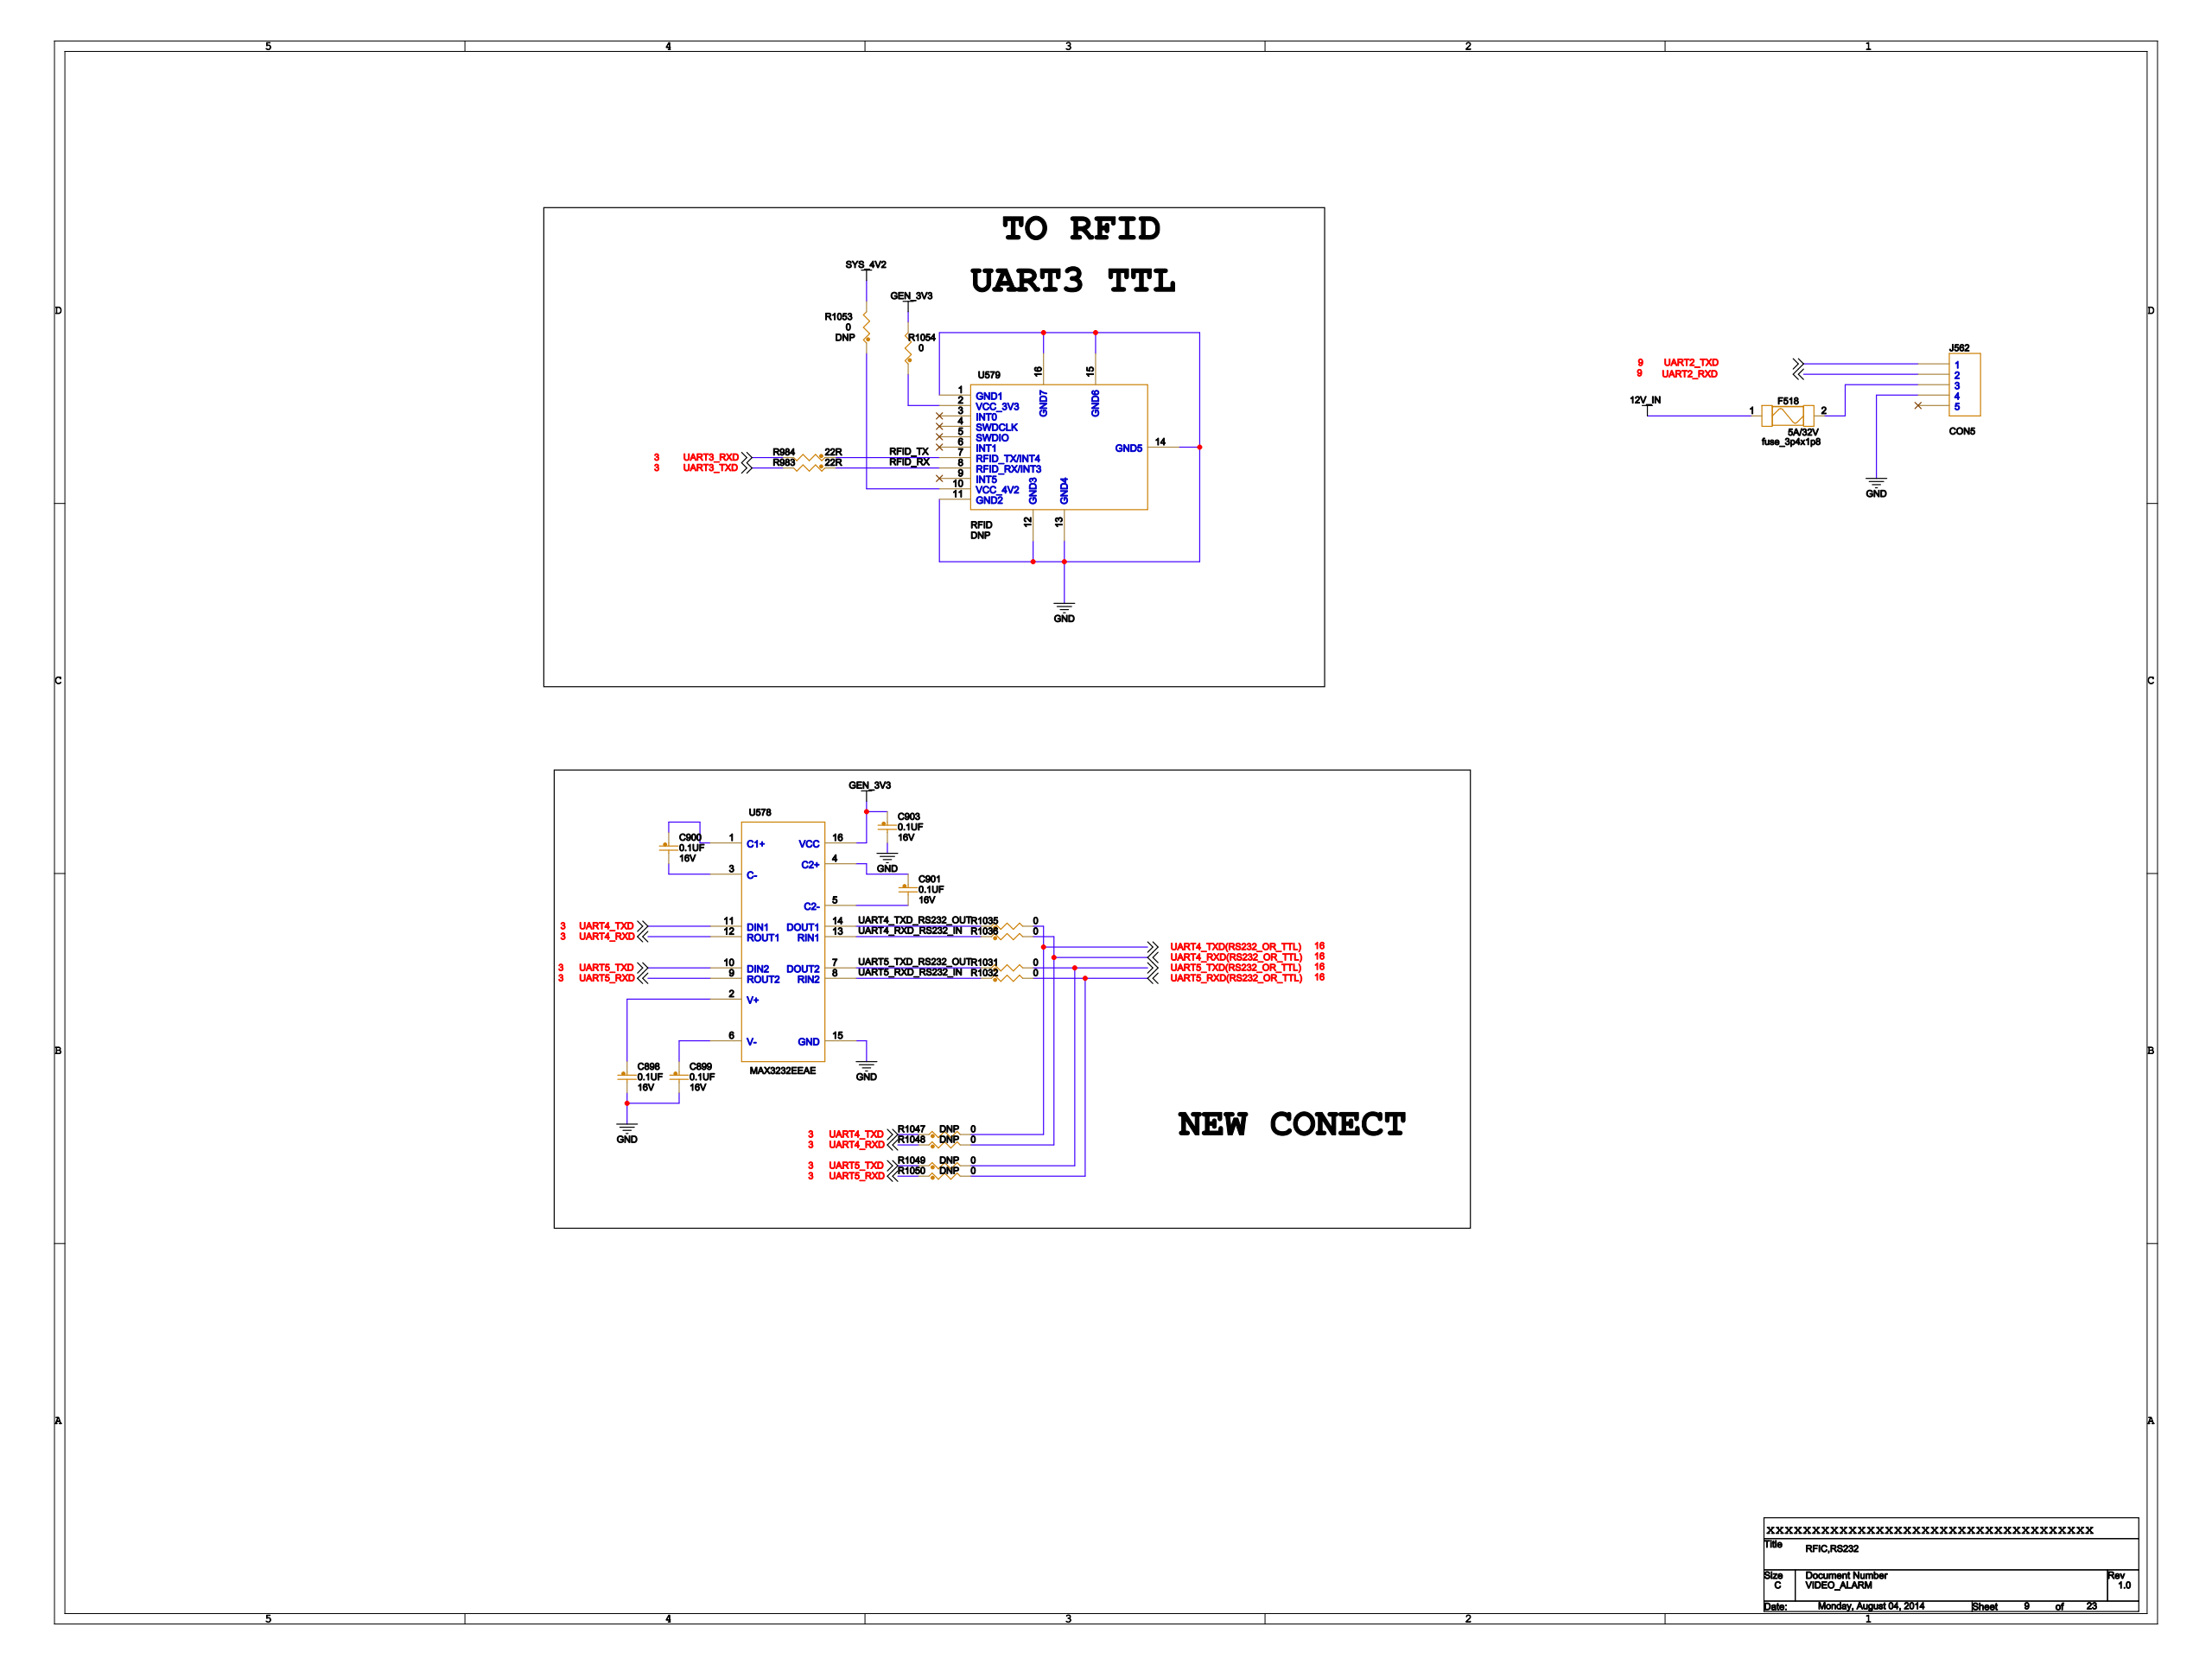Circuit board | Cadence Allegro | 994 parts | 728 nets | one sheet of the schematic
Parts on this sheet (reference | value | footprint):
C898 | 0.1UF | 0603_CC
C899 | 0.1UF | 0603_CC
C900 | 0.1UF | 0603_CC
C901 | 0.1UF | 0603_CC
C903 | 0.1UF | 0603_CC
F518 | 5A/32V | FUSE_3P4X1P8
J562 | CON5 | CON5
R983 | 22R | 0603_CC
R984 | 22R | 0603_CC
R1031 | 0 | 0603_CC
R1032 | 0 | 0603_CC
R1035 | 0 | 0603_CC
R1036 | 0 | 0603_CC
R1047 | 0 | 0603_CC
R1048 | 0 | 0603_CC
R1049 | 0 | 0603_CC
R1050 | 0 | 0603_CC
R1053 | 0 | 0805_CC
R1054 | 0 | 0805_CC
U578 | MAX3232EEAE | MAX3232-SMD1
U579 | RFID | RFID
Nets of these parts (net: part-pin ...):
GND: C898-2 C899-2 C903-2 J562-4 U578-15 U579-1 U579-11 U579-12 U579-13 U579-14 U579-15 U579-16
12V_IN: F518-1
GEN_3V3: C903-1 R1054-2 U578-16
SYS_4V2: R1053-2
N22591510: C900-1 U578-1
N22591446: C898-1 U578-2
N22591481: C900-2 U578-3
UART4_TXD_RS232_OUT: R1035-1 U578-14
N22591522: C901-1 U578-4
N22591518: C901-2 U578-5
UART4_RXD: R1036-2 R1048-1 R1048-2 U578-12
UART4_RXD_RS232_IN: R1036-1 U578-13
N22591450: C899-1 U578-6
UART5_TXD_RS232_OUT: R1031-1 U578-7
UART5_TXD: R1031-2 R1049-1 R1049-2 U578-10
UART4_TXD: R1035-2 R1047-1 R1047-2 U578-11
UART5_RXD_RS232_IN: R1032-1 U578-8
UART5_RXD: R1032-2 R1050-1 R1050-2 U578-9
UART2_RXD: J562-2
UART2_TXD: J562-1
N23025764: F518-2 J562-3
N22649533: R1054-1 U579-2
RFID_RX: R983-1 U579-8
RFID_TX: R984-1 U579-7
N22649640: R1053-1 U579-10
UART3_RXD: R984-2
UART3_TXD: R983-2